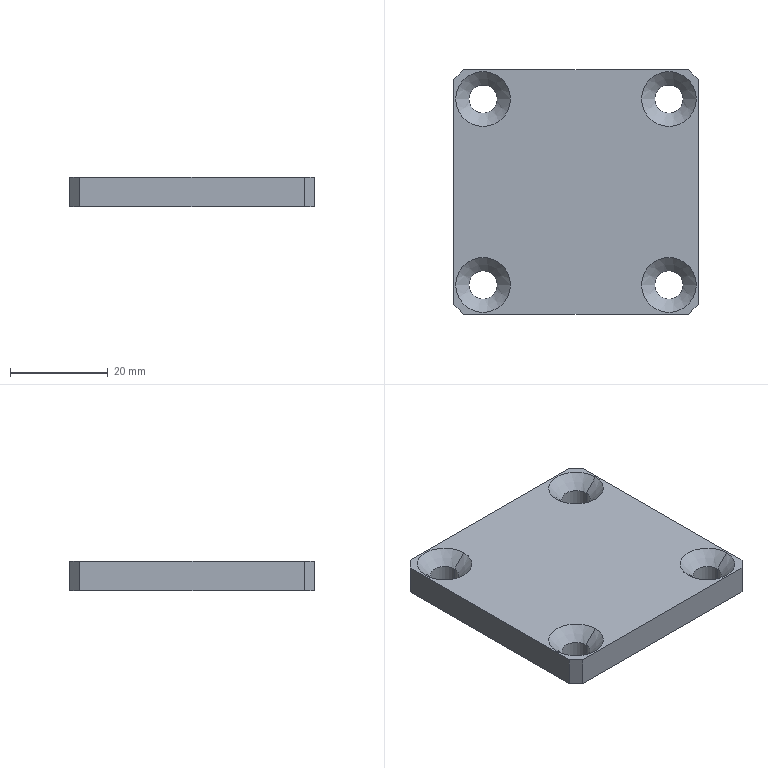Part | SolidWorks | features ICE 3, Chamfer 1, Extrusion 1, HoleWzd 1 | 1 solid | 32 faces | box 50 x 50 x 6 mm | volume 13563 mm3 | cylinder 12 | plane 12 | cone 8 | commonest cylinder face diameters 5.8 x8 33.6 x2 38.4 x2
STEP:
#1=CARTESIAN_POINT('',(-16.8,0.,-1.5));
#2=VERTEX_POINT('',#1);
#3=CARTESIAN_POINT('',(16.8,0.,-1.5));
#4=VERTEX_POINT('',#3);
#5=CARTESIAN_POINT('',(0.,0.,-1.5));
#6=DIRECTION('',(0.,0.,-1.));
#7=DIRECTION('',(-1.,0.,0.));
#8=AXIS2_PLACEMENT_3D('',#5,#6,#7);
#9=CIRCLE('',#8,16.8);
#10=EDGE_CURVE('',#2,#4,#9,.T.);
#11=ORIENTED_EDGE('',*,*,#10,.T.);
#12=CARTESIAN_POINT('',(16.8,0.,-3.));
#13=VERTEX_POINT('',#12);
#14=CARTESIAN_POINT('',(16.8,0.,-1.5));
#15=DIRECTION('',(0.,0.,-1.));
#16=VECTOR('',#15,1000.);
#17=LINE('',#14,#16);
#18=EDGE_CURVE('',#4,#13,#17,.T.);
#19=ORIENTED_EDGE('',*,*,#18,.T.);
#20=CARTESIAN_POINT('',(-16.8,0.,-3.));
#21=VERTEX_POINT('',#20);
#22=CARTESIAN_POINT('',(0.,0.,-3.));
#23=DIRECTION('',(0.,0.,-1.));
#24=DIRECTION('',(-1.,0.,0.));
#25=AXIS2_PLACEMENT_3D('',#22,#23,#24);
#26=CIRCLE('',#25,16.8);
#27=EDGE_CURVE('',#21,#13,#26,.T.);
#28=ORIENTED_EDGE('',*,*,#27,.F.);
#29=CARTESIAN_POINT('',(-16.8,0.,-1.5));
#30=DIRECTION('',(0.,0.,-1.));
#31=VECTOR('',#30,1000.);
#32=LINE('',#29,#31);
#33=EDGE_CURVE('',#2,#21,#32,.T.);
#34=ORIENTED_EDGE('',*,*,#33,.F.);
#35=EDGE_LOOP('',(#11,#19,#28,#34));
#36=FACE_OUTER_BOUND('',#35,.T.);
#37=CARTESIAN_POINT('',(0.,0.,-1.5));
#38=DIRECTION('',(0.,0.,-1.));
#39=DIRECTION('',(-1.,0.,0.));
#40=AXIS2_PLACEMENT_3D('',#37,#38,#39);
#41=CYLINDRICAL_SURFACE('',#40,16.8);
#42=ADVANCED_FACE('',(#36),#41,.T.);
#43=CARTESIAN_POINT('',(19.2,0.,-1.5));
#44=VERTEX_POINT('',#43);
#45=CARTESIAN_POINT('',(-19.2,0.,-1.5));
#46=VERTEX_POINT('',#45);
#47=CARTESIAN_POINT('',(0.,0.,-1.5));
#48=DIRECTION('',(0.,0.,-1.));
#49=DIRECTION('',(-1.,0.,0.));
#50=AXIS2_PLACEMENT_3D('',#47,#48,#49);
#51=CIRCLE('',#50,19.2);
#52=EDGE_CURVE('',#44,#46,#51,.T.);
#53=ORIENTED_EDGE('',*,*,#52,.F.);
#54=CARTESIAN_POINT('',(19.2,0.,-3.));
#55=VERTEX_POINT('',#54);
#56=CARTESIAN_POINT('',(19.2,0.,-1.5));
#57=DIRECTION('',(0.,0.,-1.));
#58=VECTOR('',#57,1000.);
#59=LINE('',#56,#58);
#60=EDGE_CURVE('',#44,#55,#59,.T.);
#61=ORIENTED_EDGE('',*,*,#60,.T.);
#62=CARTESIAN_POINT('',(-19.2,0.,-3.));
#63=VERTEX_POINT('',#62);
#64=CARTESIAN_POINT('',(0.,0.,-3.));
#65=DIRECTION('',(0.,0.,-1.));
#66=DIRECTION('',(-1.,0.,0.));
#67=AXIS2_PLACEMENT_3D('',#64,#65,#66);
#68=CIRCLE('',#67,19.2);
#69=EDGE_CURVE('',#55,#63,#68,.T.);
#70=ORIENTED_EDGE('',*,*,#69,.T.);
#71=CARTESIAN_POINT('',(-19.2,0.,-1.5));
#72=DIRECTION('',(0.,0.,-1.));
#73=VECTOR('',#72,1000.);
#74=LINE('',#71,#73);
#75=EDGE_CURVE('',#46,#63,#74,.T.);
#76=ORIENTED_EDGE('',*,*,#75,.F.);
#77=EDGE_LOOP('',(#53,#61,#70,#76));
#78=FACE_OUTER_BOUND('',#77,.T.);
#79=CARTESIAN_POINT('',(0.,0.,-1.5));
#80=DIRECTION('',(0.,0.,-1.));
#81=DIRECTION('',(-1.,0.,0.));
#82=AXIS2_PLACEMENT_3D('',#79,#80,#81);
#83=CYLINDRICAL_SURFACE('',#82,19.2);
#84=ADVANCED_FACE('',(#78),#83,.F.);
#85=CARTESIAN_POINT('',(-21.9,19.,0.3));
#86=VERTEX_POINT('',#85);
#87=CARTESIAN_POINT('',(-16.1,19.,0.3));
#88=VERTEX_POINT('',#87);
#89=CARTESIAN_POINT('',(-19.,19.,0.3));
#90=DIRECTION('',(0.,0.,1.));
#91=DIRECTION('',(1.,0.,0.));
#92=AXIS2_PLACEMENT_3D('',#89,#90,#91);
#93=CIRCLE('',#92,2.9);
#94=EDGE_CURVE('',#86,#88,#93,.T.);
#95=ORIENTED_EDGE('',*,*,#94,.F.);
#96=CARTESIAN_POINT('',(-24.6,19.,3.));
#97=VERTEX_POINT('',#96);
#98=CARTESIAN_POINT('',(-24.6,19.,3.));
#99=DIRECTION('',(-0.7071,0.,0.7071));
#100=VECTOR('',#99,1000.);
#101=LINE('',#98,#100);
#102=EDGE_CURVE('',#86,#97,#101,.T.);
#103=ORIENTED_EDGE('',*,*,#102,.T.);
#104=CARTESIAN_POINT('',(-13.4,19.,3.));
#105=VERTEX_POINT('',#104);
#106=CARTESIAN_POINT('',(-19.,19.,3.));
#107=DIRECTION('',(0.,0.,1.));
#108=DIRECTION('',(1.,0.,0.));
#109=AXIS2_PLACEMENT_3D('',#106,#107,#108);
#110=CIRCLE('',#109,5.6);
#111=EDGE_CURVE('',#97,#105,#110,.T.);
#112=ORIENTED_EDGE('',*,*,#111,.T.);
#113=CARTESIAN_POINT('',(-13.4,19.,3.));
#114=DIRECTION('',(0.7071,0.,0.7071));
#115=VECTOR('',#114,1000.);
#116=LINE('',#113,#115);
#117=EDGE_CURVE('',#88,#105,#116,.T.);
#118=ORIENTED_EDGE('',*,*,#117,.F.);
#119=EDGE_LOOP('',(#95,#103,#112,#118));
#120=FACE_OUTER_BOUND('',#119,.T.);
#121=CARTESIAN_POINT('',(-19.,19.,3.));
#122=DIRECTION('',(0.,0.,1.));
#123=DIRECTION('',(1.,0.,0.));
#124=AXIS2_PLACEMENT_3D('',#121,#122,#123);
#125=CONICAL_SURFACE('',#124,5.6,0.7854);
#126=ADVANCED_FACE('',(#120),#125,.F.);
#127=CARTESIAN_POINT('',(-21.9,19.,-3.));
#128=VERTEX_POINT('',#127);
#129=CARTESIAN_POINT('',(-16.1,19.,-3.));
#130=VERTEX_POINT('',#129);
#131=CARTESIAN_POINT('',(-19.,19.,-3.));
#132=DIRECTION('',(0.,0.,1.));
#133=DIRECTION('',(1.,0.,0.));
#134=AXIS2_PLACEMENT_3D('',#131,#132,#133);
#135=CIRCLE('',#134,2.9);
#136=EDGE_CURVE('',#128,#130,#135,.T.);
#137=ORIENTED_EDGE('',*,*,#136,.F.);
#138=CARTESIAN_POINT('',(-21.9,19.,3.));
#139=DIRECTION('',(0.,0.,1.));
#140=VECTOR('',#139,1000.);
#141=LINE('',#138,#140);
#142=EDGE_CURVE('',#128,#86,#141,.T.);
#143=ORIENTED_EDGE('',*,*,#142,.T.);
#144=ORIENTED_EDGE('',*,*,#94,.T.);
#145=CARTESIAN_POINT('',(-16.1,19.,3.));
#146=DIRECTION('',(0.,0.,1.));
#147=VECTOR('',#146,1000.);
#148=LINE('',#145,#147);
#149=EDGE_CURVE('',#130,#88,#148,.T.);
#150=ORIENTED_EDGE('',*,*,#149,.F.);
#151=EDGE_LOOP('',(#137,#143,#144,#150));
#152=FACE_OUTER_BOUND('',#151,.T.);
#153=CARTESIAN_POINT('',(-19.,19.,3.));
#154=DIRECTION('',(0.,0.,1.));
#155=DIRECTION('',(1.,0.,0.));
#156=AXIS2_PLACEMENT_3D('',#153,#154,#155);
#157=CYLINDRICAL_SURFACE('',#156,2.9);
#158=ADVANCED_FACE('',(#152),#157,.F.);
#159=CARTESIAN_POINT('',(16.1,19.,0.3));
#160=VERTEX_POINT('',#159);
#161=CARTESIAN_POINT('',(21.9,19.,0.3));
#162=VERTEX_POINT('',#161);
#163=CARTESIAN_POINT('',(19.,19.,0.3));
#164=DIRECTION('',(0.,0.,1.));
#165=DIRECTION('',(1.,0.,0.));
#166=AXIS2_PLACEMENT_3D('',#163,#164,#165);
#167=CIRCLE('',#166,2.9);
#168=EDGE_CURVE('',#160,#162,#167,.T.);
#169=ORIENTED_EDGE('',*,*,#168,.F.);
#170=CARTESIAN_POINT('',(13.4,19.,3.));
#171=VERTEX_POINT('',#170);
#172=CARTESIAN_POINT('',(13.4,19.,3.));
#173=DIRECTION('',(-0.7071,0.,0.7071));
#174=VECTOR('',#173,1000.);
#175=LINE('',#172,#174);
#176=EDGE_CURVE('',#160,#171,#175,.T.);
#177=ORIENTED_EDGE('',*,*,#176,.T.);
#178=CARTESIAN_POINT('',(24.6,19.,3.));
#179=VERTEX_POINT('',#178);
#180=CARTESIAN_POINT('',(19.,19.,3.));
#181=DIRECTION('',(0.,0.,1.));
#182=DIRECTION('',(1.,0.,0.));
#183=AXIS2_PLACEMENT_3D('',#180,#181,#182);
#184=CIRCLE('',#183,5.6);
#185=EDGE_CURVE('',#171,#179,#184,.T.);
#186=ORIENTED_EDGE('',*,*,#185,.T.);
#187=CARTESIAN_POINT('',(24.6,19.,3.));
#188=DIRECTION('',(0.7071,0.,0.7071));
#189=VECTOR('',#188,1000.);
#190=LINE('',#187,#189);
#191=EDGE_CURVE('',#162,#179,#190,.T.);
#192=ORIENTED_EDGE('',*,*,#191,.F.);
#193=EDGE_LOOP('',(#169,#177,#186,#192));
#194=FACE_OUTER_BOUND('',#193,.T.);
#195=CARTESIAN_POINT('',(19.,19.,3.));
#196=DIRECTION('',(0.,0.,1.));
#197=DIRECTION('',(1.,0.,0.));
#198=AXIS2_PLACEMENT_3D('',#195,#196,#197);
#199=CONICAL_SURFACE('',#198,5.6,0.7854);
#200=ADVANCED_FACE('',(#194),#199,.F.);
#201=CARTESIAN_POINT('',(16.1,19.,-3.));
#202=VERTEX_POINT('',#201);
#203=CARTESIAN_POINT('',(21.9,19.,-3.));
#204=VERTEX_POINT('',#203);
#205=CARTESIAN_POINT('',(19.,19.,-3.));
#206=DIRECTION('',(0.,0.,1.));
#207=DIRECTION('',(1.,0.,0.));
#208=AXIS2_PLACEMENT_3D('',#205,#206,#207);
#209=CIRCLE('',#208,2.9);
#210=EDGE_CURVE('',#202,#204,#209,.T.);
#211=ORIENTED_EDGE('',*,*,#210,.F.);
#212=CARTESIAN_POINT('',(16.1,19.,3.));
#213=DIRECTION('',(0.,0.,1.));
#214=VECTOR('',#213,1000.);
#215=LINE('',#212,#214);
#216=EDGE_CURVE('',#202,#160,#215,.T.);
#217=ORIENTED_EDGE('',*,*,#216,.T.);
#218=ORIENTED_EDGE('',*,*,#168,.T.);
#219=CARTESIAN_POINT('',(21.9,19.,3.));
#220=DIRECTION('',(0.,0.,1.));
#221=VECTOR('',#220,1000.);
#222=LINE('',#219,#221);
#223=EDGE_CURVE('',#204,#162,#222,.T.);
#224=ORIENTED_EDGE('',*,*,#223,.F.);
#225=EDGE_LOOP('',(#211,#217,#218,#224));
#226=FACE_OUTER_BOUND('',#225,.T.);
#227=CARTESIAN_POINT('',(19.,19.,3.));
#228=DIRECTION('',(0.,0.,1.));
#229=DIRECTION('',(1.,0.,0.));
#230=AXIS2_PLACEMENT_3D('',#227,#228,#229);
#231=CYLINDRICAL_SURFACE('',#230,2.9);
#232=ADVANCED_FACE('',(#226),#231,.F.);
#233=CARTESIAN_POINT('',(-21.9,-19.,0.3));
#234=VERTEX_POINT('',#233);
#235=CARTESIAN_POINT('',(-16.1,-19.,0.3));
#236=VERTEX_POINT('',#235);
#237=CARTESIAN_POINT('',(-19.,-19.,0.3));
#238=DIRECTION('',(0.,0.,1.));
#239=DIRECTION('',(1.,0.,0.));
#240=AXIS2_PLACEMENT_3D('',#237,#238,#239);
#241=CIRCLE('',#240,2.9);
#242=EDGE_CURVE('',#234,#236,#241,.T.);
#243=ORIENTED_EDGE('',*,*,#242,.F.);
#244=CARTESIAN_POINT('',(-24.6,-19.,3.));
#245=VERTEX_POINT('',#244);
#246=CARTESIAN_POINT('',(-24.6,-19.,3.));
#247=DIRECTION('',(-0.7071,0.,0.7071));
#248=VECTOR('',#247,1000.);
#249=LINE('',#246,#248);
#250=EDGE_CURVE('',#234,#245,#249,.T.);
#251=ORIENTED_EDGE('',*,*,#250,.T.);
#252=CARTESIAN_POINT('',(-13.4,-19.,3.));
#253=VERTEX_POINT('',#252);
#254=CARTESIAN_POINT('',(-19.,-19.,3.));
#255=DIRECTION('',(0.,0.,1.));
#256=DIRECTION('',(1.,0.,0.));
#257=AXIS2_PLACEMENT_3D('',#254,#255,#256);
#258=CIRCLE('',#257,5.6);
#259=EDGE_CURVE('',#245,#253,#258,.T.);
#260=ORIENTED_EDGE('',*,*,#259,.T.);
#261=CARTESIAN_POINT('',(-13.4,-19.,3.));
#262=DIRECTION('',(0.7071,0.,0.7071));
#263=VECTOR('',#262,1000.);
#264=LINE('',#261,#263);
#265=EDGE_CURVE('',#236,#253,#264,.T.);
#266=ORIENTED_EDGE('',*,*,#265,.F.);
#267=EDGE_LOOP('',(#243,#251,#260,#266));
#268=FACE_OUTER_BOUND('',#267,.T.);
#269=CARTESIAN_POINT('',(-19.,-19.,3.));
#270=DIRECTION('',(0.,0.,1.));
#271=DIRECTION('',(1.,0.,0.));
#272=AXIS2_PLACEMENT_3D('',#269,#270,#271);
#273=CONICAL_SURFACE('',#272,5.6,0.7854);
#274=ADVANCED_FACE('',(#268),#273,.F.);
#275=CARTESIAN_POINT('',(-21.9,-19.,-3.));
#276=VERTEX_POINT('',#275);
#277=CARTESIAN_POINT('',(-16.1,-19.,-3.));
#278=VERTEX_POINT('',#277);
#279=CARTESIAN_POINT('',(-19.,-19.,-3.));
#280=DIRECTION('',(0.,0.,1.));
#281=DIRECTION('',(1.,0.,0.));
#282=AXIS2_PLACEMENT_3D('',#279,#280,#281);
#283=CIRCLE('',#282,2.9);
#284=EDGE_CURVE('',#276,#278,#283,.T.);
#285=ORIENTED_EDGE('',*,*,#284,.F.);
#286=CARTESIAN_POINT('',(-21.9,-19.,3.));
#287=DIRECTION('',(0.,0.,1.));
#288=VECTOR('',#287,1000.);
#289=LINE('',#286,#288);
#290=EDGE_CURVE('',#276,#234,#289,.T.);
#291=ORIENTED_EDGE('',*,*,#290,.T.);
#292=ORIENTED_EDGE('',*,*,#242,.T.);
#293=CARTESIAN_POINT('',(-16.1,-19.,3.));
#294=DIRECTION('',(0.,0.,1.));
#295=VECTOR('',#294,1000.);
#296=LINE('',#293,#295);
#297=EDGE_CURVE('',#278,#236,#296,.T.);
#298=ORIENTED_EDGE('',*,*,#297,.F.);
#299=EDGE_LOOP('',(#285,#291,#292,#298));
#300=FACE_OUTER_BOUND('',#299,.T.);
#301=CARTESIAN_POINT('',(-19.,-19.,3.));
#302=DIRECTION('',(0.,0.,1.));
#303=DIRECTION('',(1.,0.,0.));
#304=AXIS2_PLACEMENT_3D('',#301,#302,#303);
#305=CYLINDRICAL_SURFACE('',#304,2.9);
#306=ADVANCED_FACE('',(#300),#305,.F.);
#307=CARTESIAN_POINT('',(16.1,-19.,0.3));
#308=VERTEX_POINT('',#307);
#309=CARTESIAN_POINT('',(21.9,-19.,0.3));
#310=VERTEX_POINT('',#309);
#311=CARTESIAN_POINT('',(19.,-19.,0.3));
#312=DIRECTION('',(0.,0.,1.));
#313=DIRECTION('',(1.,0.,0.));
#314=AXIS2_PLACEMENT_3D('',#311,#312,#313);
#315=CIRCLE('',#314,2.9);
#316=EDGE_CURVE('',#308,#310,#315,.T.);
#317=ORIENTED_EDGE('',*,*,#316,.F.);
#318=CARTESIAN_POINT('',(13.4,-19.,3.));
#319=VERTEX_POINT('',#318);
#320=CARTESIAN_POINT('',(13.4,-19.,3.));
#321=DIRECTION('',(-0.7071,0.,0.7071));
#322=VECTOR('',#321,1000.);
#323=LINE('',#320,#322);
#324=EDGE_CURVE('',#308,#319,#323,.T.);
#325=ORIENTED_EDGE('',*,*,#324,.T.);
#326=CARTESIAN_POINT('',(24.6,-19.,3.));
#327=VERTEX_POINT('',#326);
#328=CARTESIAN_POINT('',(19.,-19.,3.));
#329=DIRECTION('',(0.,0.,1.));
#330=DIRECTION('',(1.,0.,0.));
#331=AXIS2_PLACEMENT_3D('',#328,#329,#330);
#332=CIRCLE('',#331,5.6);
#333=EDGE_CURVE('',#319,#327,#332,.T.);
#334=ORIENTED_EDGE('',*,*,#333,.T.);
#335=CARTESIAN_POINT('',(24.6,-19.,3.));
#336=DIRECTION('',(0.7071,0.,0.7071));
#337=VECTOR('',#336,1000.);
#338=LINE('',#335,#337);
#339=EDGE_CURVE('',#310,#327,#338,.T.);
#340=ORIENTED_EDGE('',*,*,#339,.F.);
#341=EDGE_LOOP('',(#317,#325,#334,#340));
#342=FACE_OUTER_BOUND('',#341,.T.);
#343=CARTESIAN_POINT('',(19.,-19.,3.));
#344=DIRECTION('',(0.,0.,1.));
#345=DIRECTION('',(1.,0.,0.));
#346=AXIS2_PLACEMENT_3D('',#343,#344,#345);
#347=CONICAL_SURFACE('',#346,5.6,0.7854);
#348=ADVANCED_FACE('',(#342),#347,.F.);
#349=CARTESIAN_POINT('',(16.1,-19.,-3.));
#350=VERTEX_POINT('',#349);
#351=CARTESIAN_POINT('',(21.9,-19.,-3.));
#352=VERTEX_POINT('',#351);
#353=CARTESIAN_POINT('',(19.,-19.,-3.));
#354=DIRECTION('',(0.,0.,1.));
#355=DIRECTION('',(1.,0.,0.));
#356=AXIS2_PLACEMENT_3D('',#353,#354,#355);
#357=CIRCLE('',#356,2.9);
#358=EDGE_CURVE('',#350,#352,#357,.T.);
#359=ORIENTED_EDGE('',*,*,#358,.F.);
#360=CARTESIAN_POINT('',(16.1,-19.,3.));
#361=DIRECTION('',(0.,0.,1.));
#362=VECTOR('',#361,1000.);
#363=LINE('',#360,#362);
#364=EDGE_CURVE('',#350,#308,#363,.T.);
#365=ORIENTED_EDGE('',*,*,#364,.T.);
#366=ORIENTED_EDGE('',*,*,#316,.T.);
#367=CARTESIAN_POINT('',(21.9,-19.,3.));
#368=DIRECTION('',(0.,0.,1.));
#369=VECTOR('',#368,1000.);
#370=LINE('',#367,#369);
#371=EDGE_CURVE('',#352,#310,#370,.T.);
#372=ORIENTED_EDGE('',*,*,#371,.F.);
#373=EDGE_LOOP('',(#359,#365,#366,#372));
#374=FACE_OUTER_BOUND('',#373,.T.);
#375=CARTESIAN_POINT('',(19.,-19.,3.));
#376=DIRECTION('',(0.,0.,1.));
#377=DIRECTION('',(1.,0.,0.));
#378=AXIS2_PLACEMENT_3D('',#375,#376,#377);
#379=CYLINDRICAL_SURFACE('',#378,2.9);
#380=ADVANCED_FACE('',(#374),#379,.F.);
#381=CARTESIAN_POINT('',(25.,-23.,3.));
#382=VERTEX_POINT('',#381);
#383=CARTESIAN_POINT('',(25.,23.,3.));
#384=VERTEX_POINT('',#383);
#385=CARTESIAN_POINT('',(25.,-25.,3.));
#386=DIRECTION('',(0.,1.,0.));
#387=VECTOR('',#386,1000.);
#388=LINE('',#385,#387);
#389=EDGE_CURVE('',#382,#384,#388,.T.);
#390=ORIENTED_EDGE('',*,*,#389,.F.);
#391=CARTESIAN_POINT('',(25.,-23.,-3.));
#392=VERTEX_POINT('',#391);
#393=CARTESIAN_POINT('',(25.,-23.,3.));
#394=DIRECTION('',(0.,0.,-1.));
#395=VECTOR('',#394,1000.);
#396=LINE('',#393,#395);
#397=EDGE_CURVE('',#382,#392,#396,.T.);
#398=ORIENTED_EDGE('',*,*,#397,.T.);
#399=CARTESIAN_POINT('',(25.,23.,-3.));
#400=VERTEX_POINT('',#399);
#401=CARTESIAN_POINT('',(25.,-25.,-3.));
#402=DIRECTION('',(0.,1.,0.));
#403=VECTOR('',#402,1000.);
#404=LINE('',#401,#403);
#405=EDGE_CURVE('',#392,#400,#404,.T.);
#406=ORIENTED_EDGE('',*,*,#405,.T.);
#407=CARTESIAN_POINT('',(25.,23.,3.));
#408=DIRECTION('',(0.,0.,1.));
#409=VECTOR('',#408,1000.);
#410=LINE('',#407,#409);
#411=EDGE_CURVE('',#400,#384,#410,.T.);
#412=ORIENTED_EDGE('',*,*,#411,.T.);
#413=EDGE_LOOP('',(#390,#398,#406,#412));
#414=FACE_OUTER_BOUND('',#413,.T.);
#415=CARTESIAN_POINT('',(25.,-25.,3.));
#416=DIRECTION('',(-1.,0.,0.));
#417=DIRECTION('',(0.,0.,1.));
#418=AXIS2_PLACEMENT_3D('',#415,#416,#417);
#419=PLANE('',#418);
#420=ADVANCED_FACE('',(#414),#419,.F.);
#421=CARTESIAN_POINT('',(23.,25.,3.));
#422=VERTEX_POINT('',#421);
#423=CARTESIAN_POINT('',(-23.,25.,3.));
#424=VERTEX_POINT('',#423);
#425=CARTESIAN_POINT('',(-25.,25.,3.));
#426=DIRECTION('',(-1.,0.,0.));
#427=VECTOR('',#426,1000.);
#428=LINE('',#425,#427);
#429=EDGE_CURVE('',#422,#424,#428,.T.);
#430=ORIENTED_EDGE('',*,*,#429,.F.);
#431=CARTESIAN_POINT('',(23.,25.,-3.));
#432=VERTEX_POINT('',#431);
#433=CARTESIAN_POINT('',(23.,25.,3.));
#434=DIRECTION('',(0.,0.,-1.));
#435=VECTOR('',#434,1000.);
#436=LINE('',#433,#435);
#437=EDGE_CURVE('',#422,#432,#436,.T.);
#438=ORIENTED_EDGE('',*,*,#437,.T.);
#439=CARTESIAN_POINT('',(-23.,25.,-3.));
#440=VERTEX_POINT('',#439);
#441=CARTESIAN_POINT('',(-25.,25.,-3.));
#442=DIRECTION('',(-1.,0.,0.));
#443=VECTOR('',#442,1000.);
#444=LINE('',#441,#443);
#445=EDGE_CURVE('',#432,#440,#444,.T.);
#446=ORIENTED_EDGE('',*,*,#445,.T.);
#447=CARTESIAN_POINT('',(-23.,25.,3.));
#448=DIRECTION('',(0.,0.,1.));
#449=VECTOR('',#448,1000.);
#450=LINE('',#447,#449);
#451=EDGE_CURVE('',#440,#424,#450,.T.);
#452=ORIENTED_EDGE('',*,*,#451,.T.);
#453=EDGE_LOOP('',(#430,#438,#446,#452));
#454=FACE_OUTER_BOUND('',#453,.T.);
#455=CARTESIAN_POINT('',(-25.,25.,3.));
#456=DIRECTION('',(0.,-1.,0.));
#457=DIRECTION('',(0.,0.,-1.));
#458=AXIS2_PLACEMENT_3D('',#455,#456,#457);
#459=PLANE('',#458);
#460=ADVANCED_FACE('',(#454),#459,.F.);
#461=CARTESIAN_POINT('',(-25.,23.,-3.));
#462=VERTEX_POINT('',#461);
#463=CARTESIAN_POINT('',(-25.,-23.,-3.));
#464=VERTEX_POINT('',#463);
#465=CARTESIAN_POINT('',(-25.,-25.,-3.));
#466=DIRECTION('',(0.,-1.,0.));
#467=VECTOR('',#466,1000.);
#468=LINE('',#465,#467);
#469=EDGE_CURVE('',#462,#464,#468,.T.);
#470=ORIENTED_EDGE('',*,*,#469,.T.);
#471=CARTESIAN_POINT('',(-25.,-23.,3.));
#472=VERTEX_POINT('',#471);
#473=CARTESIAN_POINT('',(-25.,-23.,3.));
#474=DIRECTION('',(0.,0.,1.));
#475=VECTOR('',#474,1000.);
#476=LINE('',#473,#475);
#477=EDGE_CURVE('',#464,#472,#476,.T.);
#478=ORIENTED_EDGE('',*,*,#477,.T.);
#479=CARTESIAN_POINT('',(-25.,23.,3.));
#480=VERTEX_POINT('',#479);
#481=CARTESIAN_POINT('',(-25.,-25.,3.));
#482=DIRECTION('',(0.,-1.,0.));
#483=VECTOR('',#482,1000.);
#484=LINE('',#481,#483);
#485=EDGE_CURVE('',#480,#472,#484,.T.);
#486=ORIENTED_EDGE('',*,*,#485,.F.);
#487=CARTESIAN_POINT('',(-25.,23.,3.));
#488=DIRECTION('',(0.,0.,-1.));
#489=VECTOR('',#488,1000.);
#490=LINE('',#487,#489);
#491=EDGE_CURVE('',#480,#462,#490,.T.);
#492=ORIENTED_EDGE('',*,*,#491,.T.);
#493=EDGE_LOOP('',(#470,#478,#486,#492));
#494=FACE_OUTER_BOUND('',#493,.T.);
#495=CARTESIAN_POINT('',(-25.,-25.,3.));
#496=DIRECTION('',(1.,0.,0.));
#497=DIRECTION('',(0.,0.,-1.));
#498=AXIS2_PLACEMENT_3D('',#495,#496,#497);
#499=PLANE('',#498);
#500=ADVANCED_FACE('',(#494),#499,.F.);
#501=CARTESIAN_POINT('',(-23.,-25.,3.));
#502=VERTEX_POINT('',#501);
#503=CARTESIAN_POINT('',(23.,-25.,3.));
#504=VERTEX_POINT('',#503);
#505=CARTESIAN_POINT('',(-25.,-25.,3.));
#506=DIRECTION('',(1.,0.,0.));
#507=VECTOR('',#506,1000.);
#508=LINE('',#505,#507);
#509=EDGE_CURVE('',#502,#504,#508,.T.);
#510=ORIENTED_EDGE('',*,*,#509,.F.);
#511=CARTESIAN_POINT('',(-23.,-25.,-3.));
#512=VERTEX_POINT('',#511);
#513=CARTESIAN_POINT('',(-23.,-25.,3.));
#514=DIRECTION('',(0.,0.,-1.));
#515=VECTOR('',#514,1000.);
#516=LINE('',#513,#515);
#517=EDGE_CURVE('',#502,#512,#516,.T.);
#518=ORIENTED_EDGE('',*,*,#517,.T.);
#519=CARTESIAN_POINT('',(23.,-25.,-3.));
#520=VERTEX_POINT('',#519);
#521=CARTESIAN_POINT('',(-25.,-25.,-3.));
#522=DIRECTION('',(1.,0.,0.));
#523=VECTOR('',#522,1000.);
#524=LINE('',#521,#523);
#525=EDGE_CURVE('',#512,#520,#524,.T.);
#526=ORIENTED_EDGE('',*,*,#525,.T.);
#527=CARTESIAN_POINT('',(23.,-25.,3.));
#528=DIRECTION('',(0.,0.,1.));
#529=VECTOR('',#528,1000.);
#530=LINE('',#527,#529);
#531=EDGE_CURVE('',#520,#504,#530,.T.);
#532=ORIENTED_EDGE('',*,*,#531,.T.);
#533=EDGE_LOOP('',(#510,#518,#526,#532));
#534=FACE_OUTER_BOUND('',#533,.T.);
#535=CARTESIAN_POINT('',(-25.,-25.,3.));
#536=DIRECTION('',(0.,1.,0.));
#537=DIRECTION('',(0.,0.,1.));
#538=AXIS2_PLACEMENT_3D('',#535,#536,#537);
#539=PLANE('',#538);
#540=ADVANCED_FACE('',(#534),#539,.F.);
#541=CARTESIAN_POINT('',(-19.,19.,3.));
#542=DIRECTION('',(0.,0.,1.));
#543=DIRECTION('',(1.,0.,0.));
#544=AXIS2_PLACEMENT_3D('',#541,#542,#543);
#545=CIRCLE('',#544,5.6);
#546=EDGE_CURVE('',#105,#97,#545,.T.);
#547=ORIENTED_EDGE('',*,*,#546,.F.);
#548=ORIENTED_EDGE('',*,*,#111,.F.);
#549=EDGE_LOOP('',(#547,#548));
#550=FACE_BOUND('',#549,.T.);
#551=CARTESIAN_POINT('',(19.,19.,3.));
#552=DIRECTION('',(0.,0.,1.));
#553=DIRECTION('',(1.,0.,0.));
#554=AXIS2_PLACEMENT_3D('',#551,#552,#553);
#555=CIRCLE('',#554,5.6);
#556=EDGE_CURVE('',#179,#171,#555,.T.);
#557=ORIENTED_EDGE('',*,*,#556,.F.);
#558=ORIENTED_EDGE('',*,*,#185,.F.);
#559=EDGE_LOOP('',(#557,#558));
#560=FACE_BOUND('',#559,.T.);
#561=CARTESIAN_POINT('',(-19.,-19.,3.));
#562=DIRECTION('',(0.,0.,1.));
#563=DIRECTION('',(1.,0.,0.));
#564=AXIS2_PLACEMENT_3D('',#561,#562,#563);
#565=CIRCLE('',#564,5.6);
#566=EDGE_CURVE('',#253,#245,#565,.T.);
#567=ORIENTED_EDGE('',*,*,#566,.F.);
#568=ORIENTED_EDGE('',*,*,#259,.F.);
#569=EDGE_LOOP('',(#567,#568));
#570=FACE_BOUND('',#569,.T.);
#571=CARTESIAN_POINT('',(19.,-19.,3.));
#572=DIRECTION('',(0.,0.,1.));
#573=DIRECTION('',(1.,0.,0.));
#574=AXIS2_PLACEMENT_3D('',#571,#572,#573);
#575=CIRCLE('',#574,5.6);
#576=EDGE_CURVE('',#327,#319,#575,.T.);
#577=ORIENTED_EDGE('',*,*,#576,.F.);
#578=ORIENTED_EDGE('',*,*,#333,.F.);
#579=EDGE_LOOP('',(#577,#578));
#580=FACE_BOUND('',#579,.T.);
#581=ORIENTED_EDGE('',*,*,#485,.T.);
#582=CARTESIAN_POINT('',(-23.,-25.,3.));
#583=DIRECTION('',(0.7071,-0.7071,0.));
#584=VECTOR('',#583,1000.);
#585=LINE('',#582,#584);
#586=EDGE_CURVE('',#472,#502,#585,.T.);
#587=ORIENTED_EDGE('',*,*,#586,.T.);
#588=ORIENTED_EDGE('',*,*,#509,.T.);
#589=CARTESIAN_POINT('',(25.,-23.,3.));
#590=DIRECTION('',(0.7071,0.7071,0.));
#591=VECTOR('',#590,1000.);
#592=LINE('',#589,#591);
#593=EDGE_CURVE('',#504,#382,#592,.T.);
#594=ORIENTED_EDGE('',*,*,#593,.T.);
#595=ORIENTED_EDGE('',*,*,#389,.T.);
#596=CARTESIAN_POINT('',(23.,25.,3.));
#597=DIRECTION('',(-0.7071,0.7071,0.));
#598=VECTOR('',#597,1000.);
#599=LINE('',#596,#598);
#600=EDGE_CURVE('',#384,#422,#599,.T.);
#601=ORIENTED_EDGE('',*,*,#600,.T.);
#602=ORIENTED_EDGE('',*,*,#429,.T.);
#603=CARTESIAN_POINT('',(-25.,23.,3.));
#604=DIRECTION('',(-0.7071,-0.7071,0.));
#605=VECTOR('',#604,1000.);
#606=LINE('',#603,#605);
#607=EDGE_CURVE('',#424,#480,#606,.T.);
#608=ORIENTED_EDGE('',*,*,#607,.T.);
#609=EDGE_LOOP('',(#581,#587,#588,#594,#595,#601,#602,#608));
#610=FACE_OUTER_BOUND('',#609,.T.);
#611=CARTESIAN_POINT('',(0.,0.,3.));
#612=DIRECTION('',(0.,0.,-1.));
#613=DIRECTION('',(-1.,0.,0.));
#614=AXIS2_PLACEMENT_3D('',#611,#612,#613);
#615=PLANE('',#614);
#616=ADVANCED_FACE('',(#550,#560,#570,#580,#610),#615,.F.);
#617=CARTESIAN_POINT('',(0.,0.,-3.));
#618=DIRECTION('',(0.,0.,-1.));
#619=DIRECTION('',(-1.,0.,0.));
#620=AXIS2_PLACEMENT_3D('',#617,#618,#619);
#621=CIRCLE('',#620,19.2);
#622=EDGE_CURVE('',#63,#55,#621,.T.);
#623=ORIENTED_EDGE('',*,*,#622,.F.);
#624=ORIENTED_EDGE('',*,*,#69,.F.);
#625=EDGE_LOOP('',(#623,#624));
#626=FACE_BOUND('',#625,.T.);
#627=CARTESIAN_POINT('',(-19.,19.,-3.));
#628=DIRECTION('',(0.,0.,1.));
#629=DIRECTION('',(1.,0.,0.));
#630=AXIS2_PLACEMENT_3D('',#627,#628,#629);
#631=CIRCLE('',#630,2.9);
#632=EDGE_CURVE('',#130,#128,#631,.T.);
#633=ORIENTED_EDGE('',*,*,#632,.T.);
#634=ORIENTED_EDGE('',*,*,#136,.T.);
#635=EDGE_LOOP('',(#633,#634));
#636=FACE_BOUND('',#635,.T.);
#637=CARTESIAN_POINT('',(19.,19.,-3.));
#638=DIRECTION('',(0.,0.,1.));
#639=DIRECTION('',(1.,0.,0.));
#640=AXIS2_PLACEMENT_3D('',#637,#638,#639);
#641=CIRCLE('',#640,2.9);
#642=EDGE_CURVE('',#204,#202,#641,.T.);
#643=ORIENTED_EDGE('',*,*,#642,.T.);
#644=ORIENTED_EDGE('',*,*,#210,.T.);
#645=EDGE_LOOP('',(#643,#644));
#646=FACE_BOUND('',#645,.T.);
#647=CARTESIAN_POINT('',(-19.,-19.,-3.));
#648=DIRECTION('',(0.,0.,1.));
#649=DIRECTION('',(1.,0.,0.));
#650=AXIS2_PLACEMENT_3D('',#647,#648,#649);
#651=CIRCLE('',#650,2.9);
#652=EDGE_CURVE('',#278,#276,#651,.T.);
#653=ORIENTED_EDGE('',*,*,#652,.T.);
#654=ORIENTED_EDGE('',*,*,#284,.T.);
#655=EDGE_LOOP('',(#653,#654));
#656=FACE_BOUND('',#655,.T.);
#657=CARTESIAN_POINT('',(19.,-19.,-3.));
#658=DIRECTION('',(0.,0.,1.));
#659=DIRECTION('',(1.,0.,0.));
#660=AXIS2_PLACEMENT_3D('',#657,#658,#659);
#661=CIRCLE('',#660,2.9);
#662=EDGE_CURVE('',#352,#350,#661,.T.);
#663=ORIENTED_EDGE('',*,*,#662,.T.);
#664=ORIENTED_EDGE('',*,*,#358,.T.);
#665=EDGE_LOOP('',(#663,#664));
#666=FACE_BOUND('',#665,.T.);
#667=ORIENTED_EDGE('',*,*,#525,.F.);
#668=CARTESIAN_POINT('',(-24.,-24.,-3.));
#669=DIRECTION('',(-0.7071,0.7071,0.));
#670=VECTOR('',#669,1000.);
#671=LINE('',#668,#670);
#672=EDGE_CURVE('',#512,#464,#671,.T.);
#673=ORIENTED_EDGE('',*,*,#672,.T.);
#674=ORIENTED_EDGE('',*,*,#469,.F.);
#675=CARTESIAN_POINT('',(-24.,24.,-3.));
#676=DIRECTION('',(0.7071,0.7071,0.));
#677=VECTOR('',#676,1000.);
#678=LINE('',#675,#677);
#679=EDGE_CURVE('',#462,#440,#678,.T.);
#680=ORIENTED_EDGE('',*,*,#679,.T.);
#681=ORIENTED_EDGE('',*,*,#445,.F.);
#682=CARTESIAN_POINT('',(24.,24.,-3.));
#683=DIRECTION('',(0.7071,-0.7071,0.));
#684=VECTOR('',#683,1000.);
#685=LINE('',#682,#684);
#686=EDGE_CURVE('',#432,#400,#685,.T.);
#687=ORIENTED_EDGE('',*,*,#686,.T.);
#688=ORIENTED_EDGE('',*,*,#405,.F.);
#689=CARTESIAN_POINT('',(24.,-24.,-3.));
#690=DIRECTION('',(-0.7071,-0.7071,0.));
#691=VECTOR('',#690,1000.);
#692=LINE('',#689,#691);
#693=EDGE_CURVE('',#392,#520,#692,.T.);
#694=ORIENTED_EDGE('',*,*,#693,.T.);
#695=EDGE_LOOP('',(#667,#673,#674,#680,#681,#687,#688,#694));
#696=FACE_OUTER_BOUND('',#695,.T.);
#697=CARTESIAN_POINT('',(0.,0.,-3.));
#698=DIRECTION('',(0.,0.,-1.));
#699=DIRECTION('',(-1.,0.,0.));
#700=AXIS2_PLACEMENT_3D('',#697,#698,#699);
#701=PLANE('',#700);
#702=ADVANCED_FACE('',(#626,#636,#646,#656,#666,#696),#701,.T.);
#703=ORIENTED_EDGE('',*,*,#364,.F.);
#704=ORIENTED_EDGE('',*,*,#662,.F.);
#705=ORIENTED_EDGE('',*,*,#371,.T.);
#706=CARTESIAN_POINT('',(19.,-19.,0.3));
#707=DIRECTION('',(0.,0.,1.));
#708=DIRECTION('',(1.,0.,0.));
#709=AXIS2_PLACEMENT_3D('',#706,#707,#708);
#710=CIRCLE('',#709,2.9);
#711=EDGE_CURVE('',#310,#308,#710,.T.);
#712=ORIENTED_EDGE('',*,*,#711,.T.);
#713=EDGE_LOOP('',(#703,#704,#705,#712));
#714=FACE_OUTER_BOUND('',#713,.T.);
#715=CARTESIAN_POINT('',(19.,-19.,3.));
#716=DIRECTION('',(0.,0.,1.));
#717=DIRECTION('',(1.,0.,0.));
#718=AXIS2_PLACEMENT_3D('',#715,#716,#717);
#719=CYLINDRICAL_SURFACE('',#718,2.9);
#720=ADVANCED_FACE('',(#714),#719,.F.);
#721=ORIENTED_EDGE('',*,*,#324,.F.);
#722=ORIENTED_EDGE('',*,*,#711,.F.);
#723=ORIENTED_EDGE('',*,*,#339,.T.);
#724=ORIENTED_EDGE('',*,*,#576,.T.);
#725=EDGE_LOOP('',(#721,#722,#723,#724));
#726=FACE_OUTER_BOUND('',#725,.T.);
#727=CARTESIAN_POINT('',(19.,-19.,3.));
#728=DIRECTION('',(0.,0.,1.));
#729=DIRECTION('',(1.,0.,0.));
#730=AXIS2_PLACEMENT_3D('',#727,#728,#729);
#731=CONICAL_SURFACE('',#730,5.6,0.7854);
#732=ADVANCED_FACE('',(#726),#731,.F.);
#733=ORIENTED_EDGE('',*,*,#290,.F.);
#734=ORIENTED_EDGE('',*,*,#652,.F.);
#735=ORIENTED_EDGE('',*,*,#297,.T.);
#736=CARTESIAN_POINT('',(-19.,-19.,0.3));
#737=DIRECTION('',(0.,0.,1.));
#738=DIRECTION('',(1.,0.,0.));
#739=AXIS2_PLACEMENT_3D('',#736,#737,#738);
#740=CIRCLE('',#739,2.9);
#741=EDGE_CURVE('',#236,#234,#740,.T.);
#742=ORIENTED_EDGE('',*,*,#741,.T.);
#743=EDGE_LOOP('',(#733,#734,#735,#742));
#744=FACE_OUTER_BOUND('',#743,.T.);
#745=CARTESIAN_POINT('',(-19.,-19.,3.));
#746=DIRECTION('',(0.,0.,1.));
#747=DIRECTION('',(1.,0.,0.));
#748=AXIS2_PLACEMENT_3D('',#745,#746,#747);
#749=CYLINDRICAL_SURFACE('',#748,2.9);
#750=ADVANCED_FACE('',(#744),#749,.F.);
#751=ORIENTED_EDGE('',*,*,#250,.F.);
#752=ORIENTED_EDGE('',*,*,#741,.F.);
#753=ORIENTED_EDGE('',*,*,#265,.T.);
#754=ORIENTED_EDGE('',*,*,#566,.T.);
#755=EDGE_LOOP('',(#751,#752,#753,#754));
#756=FACE_OUTER_BOUND('',#755,.T.);
#757=CARTESIAN_POINT('',(-19.,-19.,3.));
#758=DIRECTION('',(0.,0.,1.));
#759=DIRECTION('',(1.,0.,0.));
#760=AXIS2_PLACEMENT_3D('',#757,#758,#759);
#761=CONICAL_SURFACE('',#760,5.6,0.7854);
#762=ADVANCED_FACE('',(#756),#761,.F.);
#763=ORIENTED_EDGE('',*,*,#216,.F.);
#764=ORIENTED_EDGE('',*,*,#642,.F.);
#765=ORIENTED_EDGE('',*,*,#223,.T.);
#766=CARTESIAN_POINT('',(19.,19.,0.3));
#767=DIRECTION('',(0.,0.,1.));
#768=DIRECTION('',(1.,0.,0.));
#769=AXIS2_PLACEMENT_3D('',#766,#767,#768);
#770=CIRCLE('',#769,2.9);
#771=EDGE_CURVE('',#162,#160,#770,.T.);
#772=ORIENTED_EDGE('',*,*,#771,.T.);
#773=EDGE_LOOP('',(#763,#764,#765,#772));
#774=FACE_OUTER_BOUND('',#773,.T.);
#775=CARTESIAN_POINT('',(19.,19.,3.));
#776=DIRECTION('',(0.,0.,1.));
#777=DIRECTION('',(1.,0.,0.));
#778=AXIS2_PLACEMENT_3D('',#775,#776,#777);
#779=CYLINDRICAL_SURFACE('',#778,2.9);
#780=ADVANCED_FACE('',(#774),#779,.F.);
#781=ORIENTED_EDGE('',*,*,#176,.F.);
#782=ORIENTED_EDGE('',*,*,#771,.F.);
#783=ORIENTED_EDGE('',*,*,#191,.T.);
#784=ORIENTED_EDGE('',*,*,#556,.T.);
#785=EDGE_LOOP('',(#781,#782,#783,#784));
#786=FACE_OUTER_BOUND('',#785,.T.);
#787=CARTESIAN_POINT('',(19.,19.,3.));
#788=DIRECTION('',(0.,0.,1.));
#789=DIRECTION('',(1.,0.,0.));
#790=AXIS2_PLACEMENT_3D('',#787,#788,#789);
#791=CONICAL_SURFACE('',#790,5.6,0.7854);
#792=ADVANCED_FACE('',(#786),#791,.F.);
#793=ORIENTED_EDGE('',*,*,#142,.F.);
#794=ORIENTED_EDGE('',*,*,#632,.F.);
#795=ORIENTED_EDGE('',*,*,#149,.T.);
#796=CARTESIAN_POINT('',(-19.,19.,0.3));
#797=DIRECTION('',(0.,0.,1.));
#798=DIRECTION('',(1.,0.,0.));
#799=AXIS2_PLACEMENT_3D('',#796,#797,#798);
#800=CIRCLE('',#799,2.9);
#801=EDGE_CURVE('',#88,#86,#800,.T.);
#802=ORIENTED_EDGE('',*,*,#801,.T.);
#803=EDGE_LOOP('',(#793,#794,#795,#802));
#804=FACE_OUTER_BOUND('',#803,.T.);
#805=CARTESIAN_POINT('',(-19.,19.,3.));
#806=DIRECTION('',(0.,0.,1.));
#807=DIRECTION('',(1.,0.,0.));
#808=AXIS2_PLACEMENT_3D('',#805,#806,#807);
#809=CYLINDRICAL_SURFACE('',#808,2.9);
#810=ADVANCED_FACE('',(#804),#809,.F.);
#811=ORIENTED_EDGE('',*,*,#102,.F.);
#812=ORIENTED_EDGE('',*,*,#801,.F.);
#813=ORIENTED_EDGE('',*,*,#117,.T.);
#814=ORIENTED_EDGE('',*,*,#546,.T.);
#815=EDGE_LOOP('',(#811,#812,#813,#814));
#816=FACE_OUTER_BOUND('',#815,.T.);
#817=CARTESIAN_POINT('',(-19.,19.,3.));
#818=DIRECTION('',(0.,0.,1.));
#819=DIRECTION('',(1.,0.,0.));
#820=AXIS2_PLACEMENT_3D('',#817,#818,#819);
#821=CONICAL_SURFACE('',#820,5.6,0.7854);
#822=ADVANCED_FACE('',(#816),#821,.F.);
#823=ORIENTED_EDGE('',*,*,#586,.F.);
#824=ORIENTED_EDGE('',*,*,#477,.F.);
#825=ORIENTED_EDGE('',*,*,#672,.F.);
#826=ORIENTED_EDGE('',*,*,#517,.F.);
#827=EDGE_LOOP('',(#823,#824,#825,#826));
#828=FACE_OUTER_BOUND('',#827,.T.);
#829=CARTESIAN_POINT('',(-23.,-25.,3.));
#830=DIRECTION('',(0.7071,0.7071,0.));
#831=DIRECTION('',(0.,0.,-1.));
#832=AXIS2_PLACEMENT_3D('',#829,#830,#831);
#833=PLANE('',#832);
#834=ADVANCED_FACE('',(#828),#833,.F.);
#835=ORIENTED_EDGE('',*,*,#593,.F.);
#836=ORIENTED_EDGE('',*,*,#531,.F.);
#837=ORIENTED_EDGE('',*,*,#693,.F.);
#838=ORIENTED_EDGE('',*,*,#397,.F.);
#839=EDGE_LOOP('',(#835,#836,#837,#838));
#840=FACE_OUTER_BOUND('',#839,.T.);
#841=CARTESIAN_POINT('',(25.,-23.,3.));
#842=DIRECTION('',(-0.7071,0.7071,0.));
#843=DIRECTION('',(0.,0.,-1.));
#844=AXIS2_PLACEMENT_3D('',#841,#842,#843);
#845=PLANE('',#844);
#846=ADVANCED_FACE('',(#840),#845,.F.);
#847=ORIENTED_EDGE('',*,*,#600,.F.);
#848=ORIENTED_EDGE('',*,*,#411,.F.);
#849=ORIENTED_EDGE('',*,*,#686,.F.);
#850=ORIENTED_EDGE('',*,*,#437,.F.);
#851=EDGE_LOOP('',(#847,#848,#849,#850));
#852=FACE_OUTER_BOUND('',#851,.T.);
#853=CARTESIAN_POINT('',(23.,25.,3.));
#854=DIRECTION('',(-0.7071,-0.7071,0.));
#855=DIRECTION('',(0.,0.,-1.));
#856=AXIS2_PLACEMENT_3D('',#853,#854,#855);
#857=PLANE('',#856);
#858=ADVANCED_FACE('',(#852),#857,.F.);
#859=ORIENTED_EDGE('',*,*,#607,.F.);
#860=ORIENTED_EDGE('',*,*,#451,.F.);
#861=ORIENTED_EDGE('',*,*,#679,.F.);
#862=ORIENTED_EDGE('',*,*,#491,.F.);
#863=EDGE_LOOP('',(#859,#860,#861,#862));
#864=FACE_OUTER_BOUND('',#863,.T.);
#865=CARTESIAN_POINT('',(-25.,23.,3.));
#866=DIRECTION('',(0.7071,-0.7071,0.));
#867=DIRECTION('',(0.,0.,-1.));
#868=AXIS2_PLACEMENT_3D('',#865,#866,#867);
#869=PLANE('',#868);
#870=ADVANCED_FACE('',(#864),#869,.F.);
#871=ORIENTED_EDGE('',*,*,#60,.F.);
#872=CARTESIAN_POINT('',(0.,0.,-1.5));
#873=DIRECTION('',(0.,0.,-1.));
#874=DIRECTION('',(-1.,0.,0.));
#875=AXIS2_PLACEMENT_3D('',#872,#873,#874);
#876=CIRCLE('',#875,19.2);
#877=EDGE_CURVE('',#46,#44,#876,.T.);
#878=ORIENTED_EDGE('',*,*,#877,.F.);
#879=ORIENTED_EDGE('',*,*,#75,.T.);
#880=ORIENTED_EDGE('',*,*,#622,.T.);
#881=EDGE_LOOP('',(#871,#878,#879,#880));
#882=FACE_OUTER_BOUND('',#881,.T.);
#883=CARTESIAN_POINT('',(0.,0.,-1.5));
#884=DIRECTION('',(0.,0.,-1.));
#885=DIRECTION('',(-1.,0.,0.));
#886=AXIS2_PLACEMENT_3D('',#883,#884,#885);
#887=CYLINDRICAL_SURFACE('',#886,19.2);
#888=ADVANCED_FACE('',(#882),#887,.F.);
#889=ORIENTED_EDGE('',*,*,#10,.F.);
#890=CARTESIAN_POINT('',(0.,0.,-1.5));
#891=DIRECTION('',(0.,0.,-1.));
#892=DIRECTION('',(-1.,0.,0.));
#893=AXIS2_PLACEMENT_3D('',#890,#891,#892);
#894=CIRCLE('',#893,16.8);
#895=EDGE_CURVE('',#4,#2,#894,.T.);
#896=ORIENTED_EDGE('',*,*,#895,.F.);
#897=EDGE_LOOP('',(#889,#896));
#898=FACE_BOUND('',#897,.T.);
#899=ORIENTED_EDGE('',*,*,#877,.T.);
#900=ORIENTED_EDGE('',*,*,#52,.T.);
#901=EDGE_LOOP('',(#899,#900));
#902=FACE_OUTER_BOUND('',#901,.T.);
#903=CARTESIAN_POINT('',(0.,0.,-1.5));
#904=DIRECTION('',(0.,0.,-1.));
#905=DIRECTION('',(-1.,0.,0.));
#906=AXIS2_PLACEMENT_3D('',#903,#904,#905);
#907=PLANE('',#906);
#908=ADVANCED_FACE('',(#898,#902),#907,.T.);
#909=ORIENTED_EDGE('',*,*,#18,.F.);
#910=ORIENTED_EDGE('',*,*,#895,.T.);
#911=ORIENTED_EDGE('',*,*,#33,.T.);
#912=CARTESIAN_POINT('',(0.,0.,-3.));
#913=DIRECTION('',(0.,0.,-1.));
#914=DIRECTION('',(-1.,0.,0.));
#915=AXIS2_PLACEMENT_3D('',#912,#913,#914);
#916=CIRCLE('',#915,16.8);
#917=EDGE_CURVE('',#13,#21,#916,.T.);
#918=ORIENTED_EDGE('',*,*,#917,.F.);
#919=EDGE_LOOP('',(#909,#910,#911,#918));
#920=FACE_OUTER_BOUND('',#919,.T.);
#921=CARTESIAN_POINT('',(0.,0.,-1.5));
#922=DIRECTION('',(0.,0.,-1.));
#923=DIRECTION('',(-1.,0.,0.));
#924=AXIS2_PLACEMENT_3D('',#921,#922,#923);
#925=CYLINDRICAL_SURFACE('',#924,16.8);
#926=ADVANCED_FACE('',(#920),#925,.T.);
#927=ORIENTED_EDGE('',*,*,#27,.T.);
#928=ORIENTED_EDGE('',*,*,#917,.T.);
#929=EDGE_LOOP('',(#927,#928));
#930=FACE_OUTER_BOUND('',#929,.T.);
#931=CARTESIAN_POINT('',(0.,0.,-3.));
#932=DIRECTION('',(0.,0.,-1.));
#933=DIRECTION('',(-1.,0.,0.));
#934=AXIS2_PLACEMENT_3D('',#931,#932,#933);
#935=PLANE('',#934);
#936=ADVANCED_FACE('',(#930),#935,.T.);
#937=CLOSED_SHELL('',(#42,#84,#126,#158,#200,#232,#274,#306,#348,#380,#420,#460,#500,#540,#616,#702,#720,#732,#750,#762,#780,#792,#810,#822,#834,#846,#858,#870,#888,#908,#926,#936));
#938=MANIFOLD_SOLID_BREP('',#937);
#939=CARTESIAN_POINT('',(0.,0.,0.));
#940=DIRECTION('',(0.,0.,1.));
#941=DIRECTION('',(1.,0.,0.));
#942=AXIS2_PLACEMENT_3D('',#939,#940,#941);
#943=(LENGTH_UNIT()NAMED_UNIT(*)SI_UNIT(.MILLI.,.METRE.));
#944=UNCERTAINTY_MEASURE_WITH_UNIT(LENGTH_MEASURE(0.00001),#943,'','');
#945=(NAMED_UNIT(*)PLANE_ANGLE_UNIT()SI_UNIT($,.RADIAN.));
#946=(NAMED_UNIT(*)SI_UNIT($,.STERADIAN.)SOLID_ANGLE_UNIT());
#947=(GEOMETRIC_REPRESENTATION_CONTEXT(3)GLOBAL_UNCERTAINTY_ASSIGNED_CONTEXT((#944))GLOBAL_UNIT_ASSIGNED_CONTEXT((#943,#945,#946))REPRESENTATION_CONTEXT('',''));
#948=ADVANCED_BREP_SHAPE_REPRESENTATION('',(#938,#942),#947);